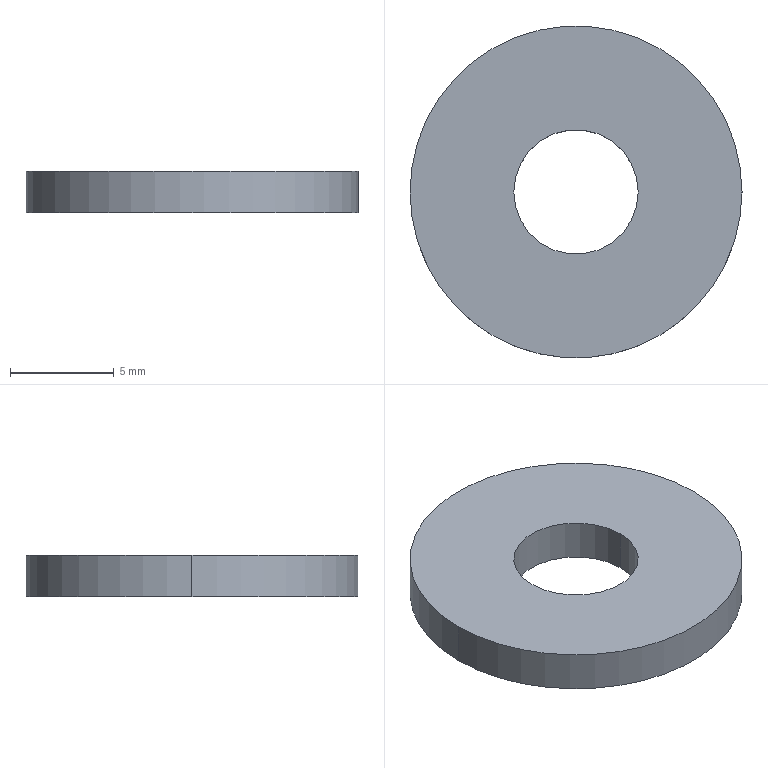Part | SolidWorks | features Extrusion 1 | 1 solid | 6 faces | box 16 x 16 x 2 mm | volume 345.575 mm3 | cylinder 4 | plane 2 | commonest cylinder face diameters 6 x2 16 x2
STEP:
#1=CARTESIAN_POINT('',(-3.,0.,2.));
#2=VERTEX_POINT('',#1);
#3=CARTESIAN_POINT('',(3.,0.,2.));
#4=VERTEX_POINT('',#3);
#5=CARTESIAN_POINT('',(0.,0.,2.));
#6=DIRECTION('',(0.,0.,1.));
#7=DIRECTION('',(1.,0.,0.));
#8=AXIS2_PLACEMENT_3D('',#5,#6,#7);
#9=CIRCLE('',#8,3.);
#10=EDGE_CURVE('',#2,#4,#9,.T.);
#11=ORIENTED_EDGE('',*,*,#10,.T.);
#12=CARTESIAN_POINT('',(3.,0.,0.));
#13=VERTEX_POINT('',#12);
#14=CARTESIAN_POINT('',(3.,0.,2.));
#15=DIRECTION('',(0.,0.,-1.));
#16=VECTOR('',#15,1000.);
#17=LINE('',#14,#16);
#18=EDGE_CURVE('',#4,#13,#17,.T.);
#19=ORIENTED_EDGE('',*,*,#18,.T.);
#20=CARTESIAN_POINT('',(-3.,0.,0.));
#21=VERTEX_POINT('',#20);
#22=CARTESIAN_POINT('',(0.,0.,0.));
#23=DIRECTION('',(0.,0.,1.));
#24=DIRECTION('',(1.,0.,0.));
#25=AXIS2_PLACEMENT_3D('',#22,#23,#24);
#26=CIRCLE('',#25,3.);
#27=EDGE_CURVE('',#21,#13,#26,.T.);
#28=ORIENTED_EDGE('',*,*,#27,.F.);
#29=CARTESIAN_POINT('',(-3.,0.,2.));
#30=DIRECTION('',(0.,0.,-1.));
#31=VECTOR('',#30,1000.);
#32=LINE('',#29,#31);
#33=EDGE_CURVE('',#2,#21,#32,.T.);
#34=ORIENTED_EDGE('',*,*,#33,.F.);
#35=EDGE_LOOP('',(#11,#19,#28,#34));
#36=FACE_OUTER_BOUND('',#35,.T.);
#37=CARTESIAN_POINT('',(0.,0.,2.));
#38=DIRECTION('',(0.,0.,-1.));
#39=DIRECTION('',(-1.,0.,0.));
#40=AXIS2_PLACEMENT_3D('',#37,#38,#39);
#41=CYLINDRICAL_SURFACE('',#40,3.);
#42=ADVANCED_FACE('',(#36),#41,.F.);
#43=CARTESIAN_POINT('',(8.,0.,2.));
#44=VERTEX_POINT('',#43);
#45=CARTESIAN_POINT('',(-8.,0.,2.));
#46=VERTEX_POINT('',#45);
#47=CARTESIAN_POINT('',(0.,0.,2.));
#48=DIRECTION('',(0.,0.,1.));
#49=DIRECTION('',(1.,0.,0.));
#50=AXIS2_PLACEMENT_3D('',#47,#48,#49);
#51=CIRCLE('',#50,8.);
#52=EDGE_CURVE('',#44,#46,#51,.T.);
#53=ORIENTED_EDGE('',*,*,#52,.F.);
#54=CARTESIAN_POINT('',(8.,0.,0.));
#55=VERTEX_POINT('',#54);
#56=CARTESIAN_POINT('',(8.,0.,2.));
#57=DIRECTION('',(0.,0.,-1.));
#58=VECTOR('',#57,1000.);
#59=LINE('',#56,#58);
#60=EDGE_CURVE('',#44,#55,#59,.T.);
#61=ORIENTED_EDGE('',*,*,#60,.T.);
#62=CARTESIAN_POINT('',(-8.,0.,0.));
#63=VERTEX_POINT('',#62);
#64=CARTESIAN_POINT('',(0.,0.,0.));
#65=DIRECTION('',(0.,0.,1.));
#66=DIRECTION('',(1.,0.,0.));
#67=AXIS2_PLACEMENT_3D('',#64,#65,#66);
#68=CIRCLE('',#67,8.);
#69=EDGE_CURVE('',#55,#63,#68,.T.);
#70=ORIENTED_EDGE('',*,*,#69,.T.);
#71=CARTESIAN_POINT('',(-8.,0.,2.));
#72=DIRECTION('',(0.,0.,-1.));
#73=VECTOR('',#72,1000.);
#74=LINE('',#71,#73);
#75=EDGE_CURVE('',#46,#63,#74,.T.);
#76=ORIENTED_EDGE('',*,*,#75,.F.);
#77=EDGE_LOOP('',(#53,#61,#70,#76));
#78=FACE_OUTER_BOUND('',#77,.T.);
#79=CARTESIAN_POINT('',(0.,0.,2.));
#80=DIRECTION('',(0.,0.,-1.));
#81=DIRECTION('',(-1.,0.,0.));
#82=AXIS2_PLACEMENT_3D('',#79,#80,#81);
#83=CYLINDRICAL_SURFACE('',#82,8.);
#84=ADVANCED_FACE('',(#78),#83,.T.);
#85=CARTESIAN_POINT('',(0.,0.,2.));
#86=DIRECTION('',(0.,0.,1.));
#87=DIRECTION('',(1.,0.,0.));
#88=AXIS2_PLACEMENT_3D('',#85,#86,#87);
#89=CIRCLE('',#88,8.);
#90=EDGE_CURVE('',#46,#44,#89,.T.);
#91=ORIENTED_EDGE('',*,*,#90,.T.);
#92=ORIENTED_EDGE('',*,*,#52,.T.);
#93=EDGE_LOOP('',(#91,#92));
#94=FACE_OUTER_BOUND('',#93,.T.);
#95=ORIENTED_EDGE('',*,*,#10,.F.);
#96=CARTESIAN_POINT('',(0.,0.,2.));
#97=DIRECTION('',(0.,0.,1.));
#98=DIRECTION('',(1.,0.,0.));
#99=AXIS2_PLACEMENT_3D('',#96,#97,#98);
#100=CIRCLE('',#99,3.);
#101=EDGE_CURVE('',#4,#2,#100,.T.);
#102=ORIENTED_EDGE('',*,*,#101,.F.);
#103=EDGE_LOOP('',(#95,#102));
#104=FACE_BOUND('',#103,.T.);
#105=CARTESIAN_POINT('',(0.,0.,2.));
#106=DIRECTION('',(0.,0.,1.));
#107=DIRECTION('',(1.,0.,0.));
#108=AXIS2_PLACEMENT_3D('',#105,#106,#107);
#109=PLANE('',#108);
#110=ADVANCED_FACE('',(#94,#104),#109,.T.);
#111=CARTESIAN_POINT('',(0.,0.,0.));
#112=DIRECTION('',(0.,0.,1.));
#113=DIRECTION('',(1.,0.,0.));
#114=AXIS2_PLACEMENT_3D('',#111,#112,#113);
#115=CIRCLE('',#114,8.);
#116=EDGE_CURVE('',#63,#55,#115,.T.);
#117=ORIENTED_EDGE('',*,*,#116,.F.);
#118=ORIENTED_EDGE('',*,*,#69,.F.);
#119=EDGE_LOOP('',(#117,#118));
#120=FACE_OUTER_BOUND('',#119,.T.);
#121=ORIENTED_EDGE('',*,*,#27,.T.);
#122=CARTESIAN_POINT('',(0.,0.,0.));
#123=DIRECTION('',(0.,0.,1.));
#124=DIRECTION('',(1.,0.,0.));
#125=AXIS2_PLACEMENT_3D('',#122,#123,#124);
#126=CIRCLE('',#125,3.);
#127=EDGE_CURVE('',#13,#21,#126,.T.);
#128=ORIENTED_EDGE('',*,*,#127,.T.);
#129=EDGE_LOOP('',(#121,#128));
#130=FACE_BOUND('',#129,.T.);
#131=CARTESIAN_POINT('',(0.,0.,0.));
#132=DIRECTION('',(0.,0.,1.));
#133=DIRECTION('',(1.,0.,0.));
#134=AXIS2_PLACEMENT_3D('',#131,#132,#133);
#135=PLANE('',#134);
#136=ADVANCED_FACE('',(#120,#130),#135,.F.);
#137=ORIENTED_EDGE('',*,*,#60,.F.);
#138=ORIENTED_EDGE('',*,*,#90,.F.);
#139=ORIENTED_EDGE('',*,*,#75,.T.);
#140=ORIENTED_EDGE('',*,*,#116,.T.);
#141=EDGE_LOOP('',(#137,#138,#139,#140));
#142=FACE_OUTER_BOUND('',#141,.T.);
#143=CARTESIAN_POINT('',(0.,0.,2.));
#144=DIRECTION('',(0.,0.,-1.));
#145=DIRECTION('',(-1.,0.,0.));
#146=AXIS2_PLACEMENT_3D('',#143,#144,#145);
#147=CYLINDRICAL_SURFACE('',#146,8.);
#148=ADVANCED_FACE('',(#142),#147,.T.);
#149=ORIENTED_EDGE('',*,*,#18,.F.);
#150=ORIENTED_EDGE('',*,*,#101,.T.);
#151=ORIENTED_EDGE('',*,*,#33,.T.);
#152=ORIENTED_EDGE('',*,*,#127,.F.);
#153=EDGE_LOOP('',(#149,#150,#151,#152));
#154=FACE_OUTER_BOUND('',#153,.T.);
#155=CARTESIAN_POINT('',(0.,0.,2.));
#156=DIRECTION('',(0.,0.,-1.));
#157=DIRECTION('',(-1.,0.,0.));
#158=AXIS2_PLACEMENT_3D('',#155,#156,#157);
#159=CYLINDRICAL_SURFACE('',#158,3.);
#160=ADVANCED_FACE('',(#154),#159,.F.);
#161=CLOSED_SHELL('',(#42,#84,#110,#136,#148,#160));
#162=MANIFOLD_SOLID_BREP('',#161);
#163=CARTESIAN_POINT('',(0.,0.,0.));
#164=DIRECTION('',(0.,0.,1.));
#165=DIRECTION('',(1.,0.,0.));
#166=AXIS2_PLACEMENT_3D('',#163,#164,#165);
#167=(LENGTH_UNIT()NAMED_UNIT(*)SI_UNIT(.MILLI.,.METRE.));
#168=UNCERTAINTY_MEASURE_WITH_UNIT(LENGTH_MEASURE(0.00001),#167,'','');
#169=(NAMED_UNIT(*)PLANE_ANGLE_UNIT()SI_UNIT($,.RADIAN.));
#170=(NAMED_UNIT(*)SI_UNIT($,.STERADIAN.)SOLID_ANGLE_UNIT());
#171=(GEOMETRIC_REPRESENTATION_CONTEXT(3)GLOBAL_UNCERTAINTY_ASSIGNED_CONTEXT((#168))GLOBAL_UNIT_ASSIGNED_CONTEXT((#167,#169,#170))REPRESENTATION_CONTEXT('',''));
#172=ADVANCED_BREP_SHAPE_REPRESENTATION('',(#162,#166),#171);